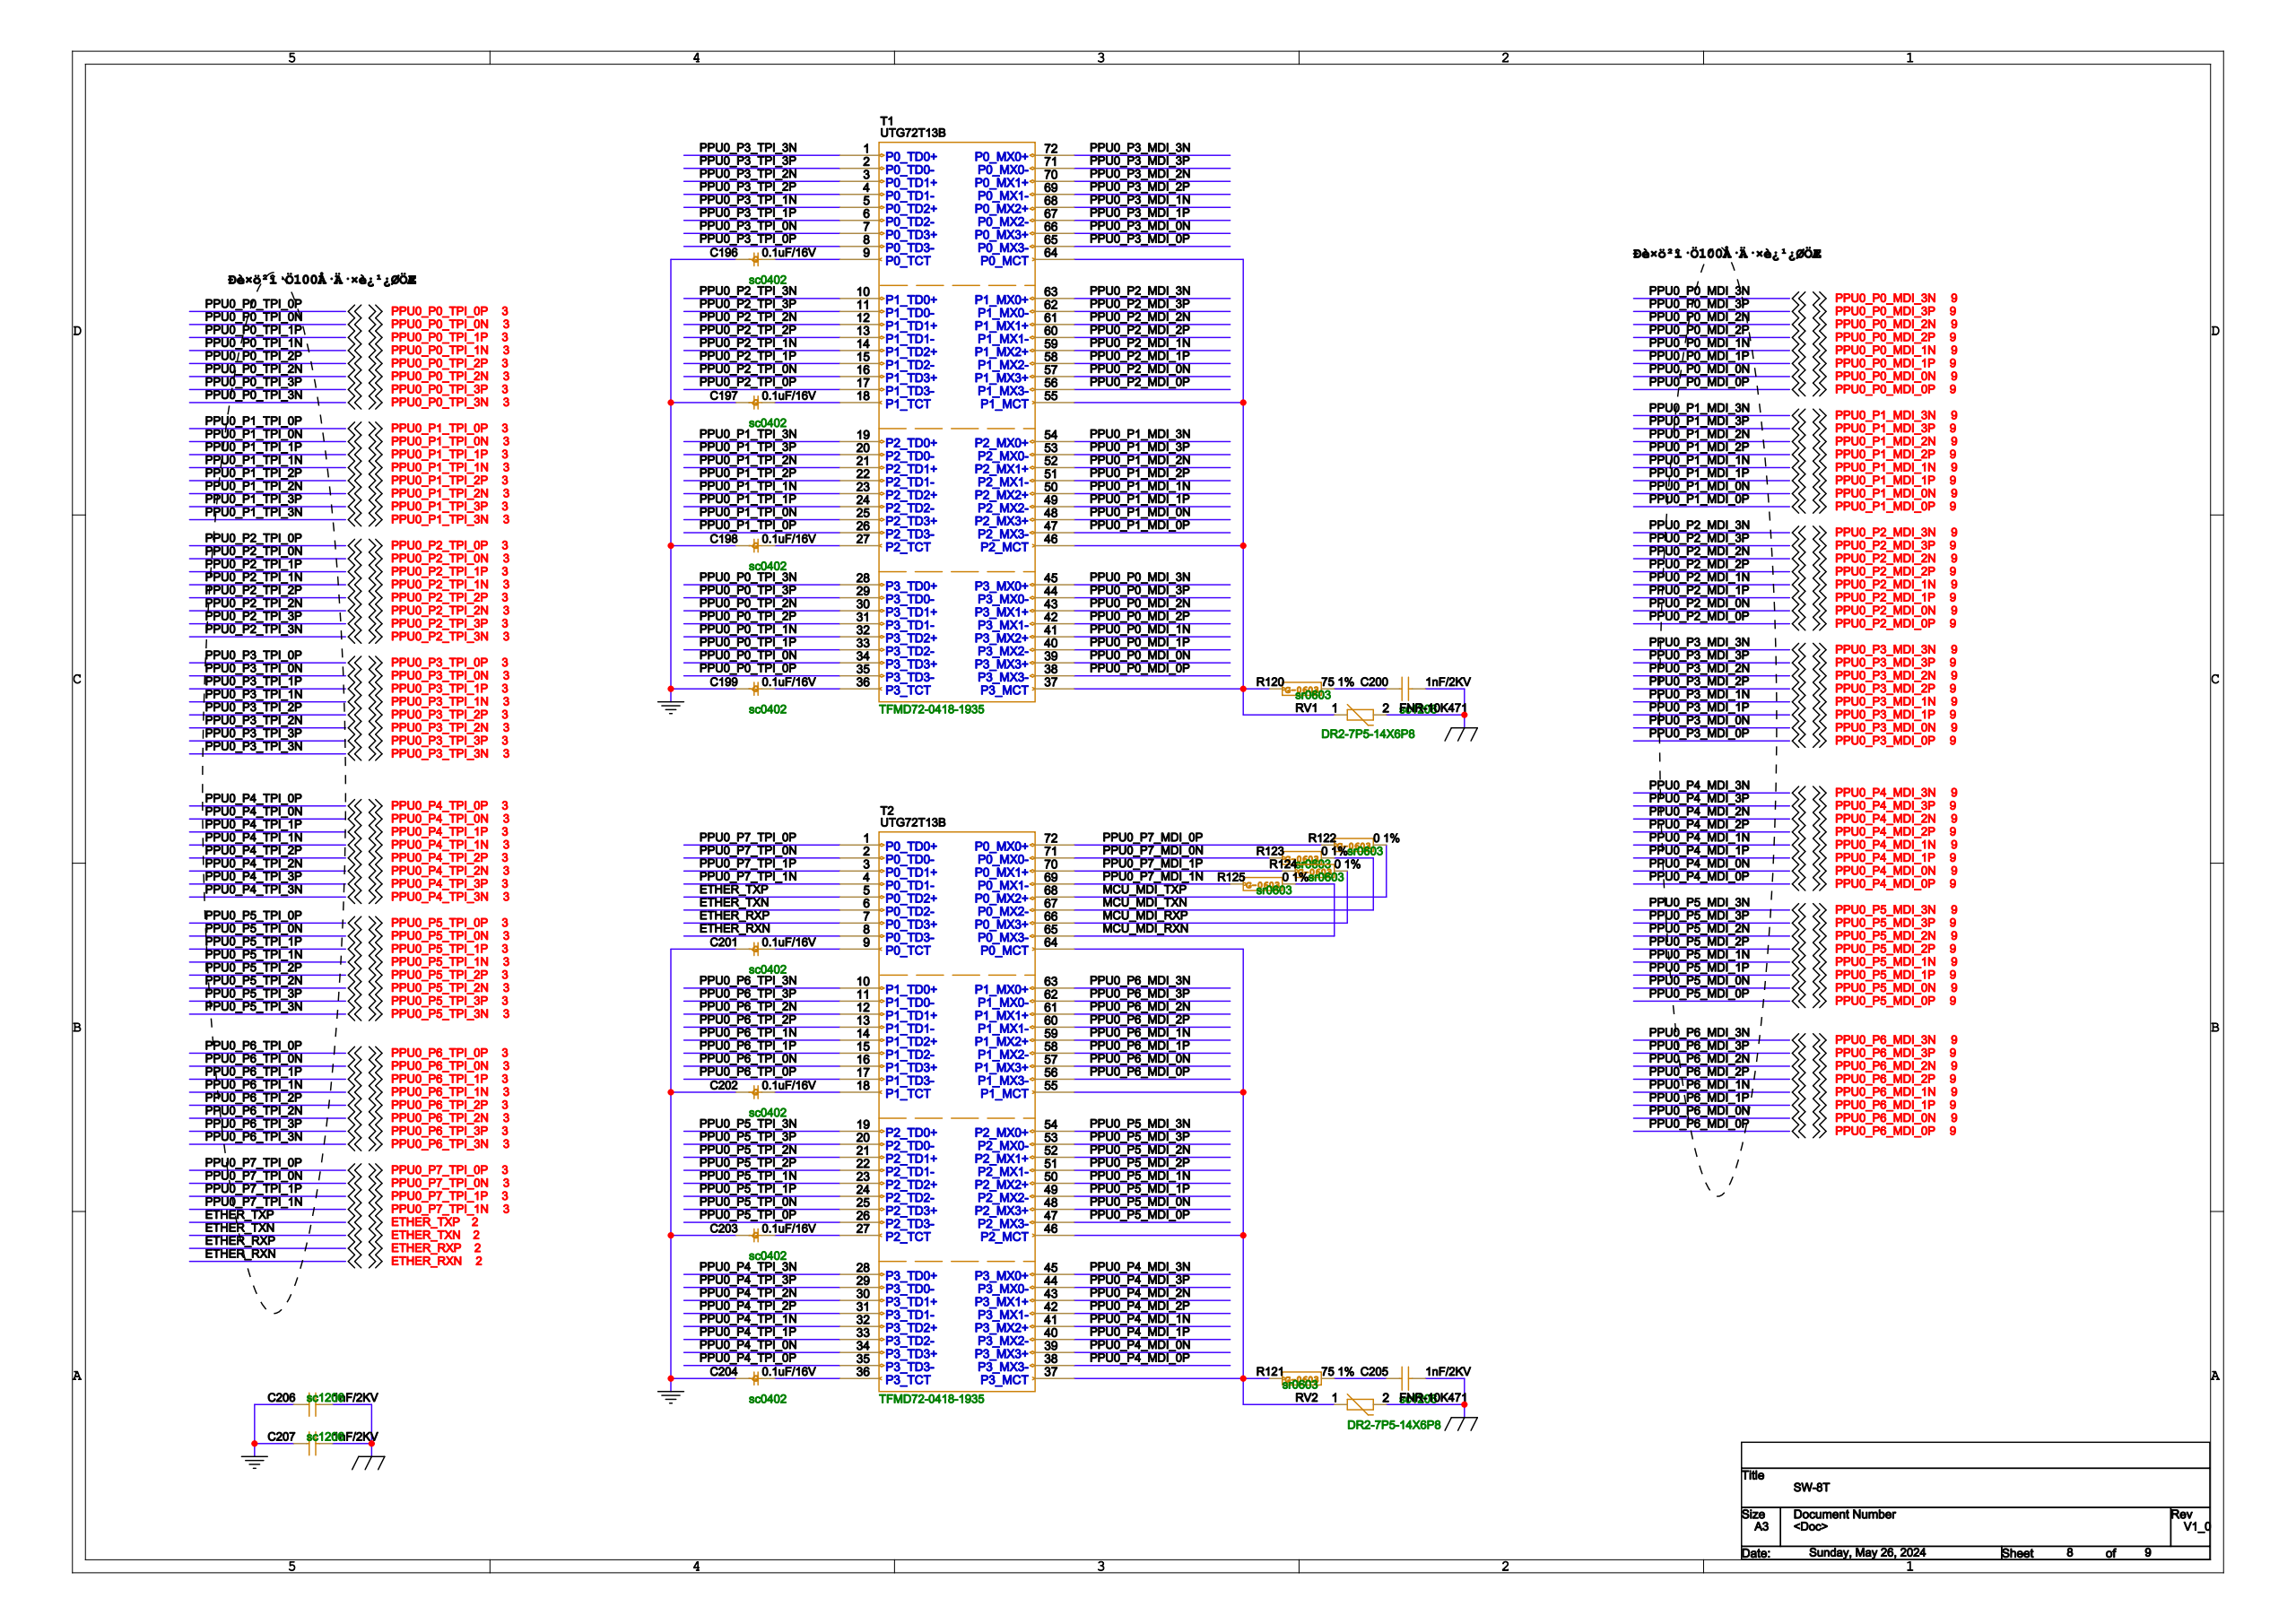Circuit board | Cadence Allegro | 399 parts | 387 nets | one sheet of the schematic
Parts on this sheet (reference | value | footprint):
C196 | 0.1uF/16V | SC0402
C197 | 0.1uF/16V | SC0402
C198 | 0.1uF/16V | SC0402
C199 | 0.1uF/16V | SC0402
C200 | 1nF/2KV | SC1206
C201 | 0.1uF/16V | SC0402
C202 | 0.1uF/16V | SC0402
C203 | 0.1uF/16V | SC0402
C204 | 0.1uF/16V | SC0402
C205 | 1nF/2KV | SC1206
C206 | 1nF/2KV | SC1206
C207 | 1nF/2KV | SC1206
R120 | 75 1% | SR0603
R121 | 75 1% | SR0603
R122 | 0 1% | SR0603
R123 | 0 1% | SR0603
R124 | 0 1% | SR0603
R125 | 0 1% | SR0603
RV1 | FNR-10K471 | DR2-7P5-14X6P8
RV2 | FNR-10K471 | DR2-7P5-14X6P8
T1 | UTG72T13B | TFMD72-0418-1935
T2 | UTG72T13B | TFMD72-0418-1935
Nets of these parts (net: part-pin ...):
PPU0_P7_MDI_0P: R122-1 T2-72
MCU_MDI_TXP: R122-2 T2-68
PPU0_P7_MDI_0N: R123-1 T2-71
MCU_MDI_TXN: R123-2 T2-67
PPU0_P7_MDI_1P: R124-1 T2-70
MCU_MDI_RXP: R124-2 T2-66
PPU0_P7_MDI_1N: R125-1 T2-69
MCU_MDI_RXN: R125-2 T2-65
GND: C196-1 C197-1 C198-1 C199-1 C201-1 C202-1 C203-1 C204-1 C206-1 C207-1
N17701580: C196-2 T1-9
N17701582: C197-2 T1-18
N17701576: C198-2 T1-27
N17701578: C199-2 T1-36
N17757693: C201-2 T2-9
N17757337: C202-2 T2-18
N17757335: C203-2 T2-27
N17757333: C204-2 T2-36
GND_EARTH: C200-2 C205-2 C206-2 C207-2 RV1-2 RV2-2
N17701628: C200-1 R120-2
N17757449: C205-1 R121-2
ETHER_TXP: T2-5
ETHER_TXN: T2-6
ETHER_RXP: T2-7
ETHER_RXN: T2-8
PPU0_P5_MDI_0N: T2-48
PPU0_P5_MDI_2N: T2-52
PPU0_P5_MDI_0P: T2-47
PPU0_P5_MDI_1N: T2-50
PPU0_P5_MDI_2P: T2-51
PPU0_P5_MDI_3N: T2-54
PPU0_P5_MDI_1P: T2-49
PPU0_P5_MDI_3P: T2-53
PPU0_P4_MDI_0N: T2-39
PPU0_P4_MDI_2N: T2-43
PPU0_P6_MDI_0N: T2-57
PPU0_P6_MDI_2N: T2-61
PPU0_P4_MDI_0P: T2-38
PPU0_P4_MDI_1N: T2-41
PPU0_P4_MDI_2P: T2-42
PPU0_P4_MDI_3N: T2-45
PPU0_P6_MDI_0P: T2-56
PPU0_P6_MDI_1N: T2-59
PPU0_P6_MDI_2P: T2-60
PPU0_P6_MDI_3N: T2-63
PPU0_P4_MDI_1P: T2-40
PPU0_P4_MDI_3P: T2-44
PPU0_P6_MDI_1P: T2-58
PPU0_P6_MDI_3P: T2-62
PPU0_P1_MDI_2N: T1-52
PPU0_P3_MDI_0N: T1-66
PPU0_P3_MDI_2N: T1-70
PPU0_P1_MDI_0N: T1-48
PPU0_P1_MDI_1N: T1-50
PPU0_P1_MDI_2P: T1-51
PPU0_P1_MDI_3N: T1-54
PPU0_P3_MDI_0P: T1-65
PPU0_P3_MDI_1N: T1-68
PPU0_P3_MDI_2P: T1-69
PPU0_P3_MDI_3N: T1-72
PPU0_P1_MDI_0P: T1-47
PPU0_P1_MDI_1P: T1-49
PPU0_P1_MDI_3P: T1-53
PPU0_P3_MDI_1P: T1-67
PPU0_P3_MDI_3P: T1-71
PPU0_P0_MDI_2N: T1-43
PPU0_P2_MDI_0N: T1-57
PPU0_P2_MDI_2N: T1-61
PPU0_P0_MDI_0N: T1-39
PPU0_P0_MDI_1N: T1-41
PPU0_P0_MDI_2P: T1-42
PPU0_P0_MDI_3N: T1-45
PPU0_P2_MDI_0P: T1-56
PPU0_P2_MDI_1N: T1-59
PPU0_P2_MDI_2P: T1-60
PPU0_P2_MDI_3N: T1-63
PPU0_P0_MDI_0P: T1-38
PPU0_P0_MDI_1P: T1-40
PPU0_P0_MDI_3P: T1-44
PPU0_P2_MDI_1P: T1-58
PPU0_P2_MDI_3P: T1-62
N17701608: R120-1 RV1-1 T1-37 T1-46 T1-55 T1-64
N17757409: R121-1 RV2-1 T2-37 T2-46 T2-55 T2-64
PPU0_P3_TPI_3N: T1-1
PPU0_P3_TPI_3P: T1-2
PPU0_P3_TPI_2N: T1-3
PPU0_P3_TPI_2P: T1-4
PPU0_P3_TPI_1N: T1-5
PPU0_P3_TPI_1P: T1-6
PPU0_P3_TPI_0N: T1-7
PPU0_P3_TPI_0P: T1-8
PPU0_P2_TPI_3N: T1-10
PPU0_P2_TPI_3P: T1-11
PPU0_P2_TPI_2N: T1-12
PPU0_P2_TPI_2P: T1-13
PPU0_P2_TPI_1N: T1-14
PPU0_P2_TPI_1P: T1-15
PPU0_P2_TPI_0N: T1-16
PPU0_P2_TPI_0P: T1-17
PPU0_P1_TPI_3N: T1-19
PPU0_P1_TPI_3P: T1-20
PPU0_P1_TPI_2N: T1-21
PPU0_P1_TPI_2P: T1-22
PPU0_P1_TPI_1N: T1-23
PPU0_P1_TPI_1P: T1-24
PPU0_P1_TPI_0N: T1-25
PPU0_P1_TPI_0P: T1-26
PPU0_P0_TPI_3N: T1-28
PPU0_P0_TPI_3P: T1-29
PPU0_P0_TPI_2N: T1-30
PPU0_P0_TPI_2P: T1-31
PPU0_P0_TPI_1N: T1-32
PPU0_P0_TPI_1P: T1-33
PPU0_P0_TPI_0N: T1-34
PPU0_P0_TPI_0P: T1-35
PPU0_P7_TPI_0P: T2-1
PPU0_P7_TPI_0N: T2-2
PPU0_P7_TPI_1P: T2-3
PPU0_P7_TPI_1N: T2-4
PPU0_P6_TPI_3N: T2-10
PPU0_P6_TPI_3P: T2-11
PPU0_P6_TPI_2N: T2-12
PPU0_P6_TPI_2P: T2-13
PPU0_P6_TPI_1N: T2-14
PPU0_P6_TPI_1P: T2-15
PPU0_P6_TPI_0N: T2-16
PPU0_P6_TPI_0P: T2-17
PPU0_P5_TPI_3N: T2-19
PPU0_P5_TPI_3P: T2-20
PPU0_P5_TPI_2N: T2-21
PPU0_P5_TPI_2P: T2-22
PPU0_P5_TPI_1N: T2-23
PPU0_P5_TPI_1P: T2-24
PPU0_P5_TPI_0N: T2-25
PPU0_P5_TPI_0P: T2-26
PPU0_P4_TPI_3N: T2-28
PPU0_P4_TPI_3P: T2-29
PPU0_P4_TPI_2N: T2-30
PPU0_P4_TPI_2P: T2-31
PPU0_P4_TPI_1N: T2-32
PPU0_P4_TPI_1P: T2-33
PPU0_P4_TPI_0N: T2-34
PPU0_P4_TPI_0P: T2-35